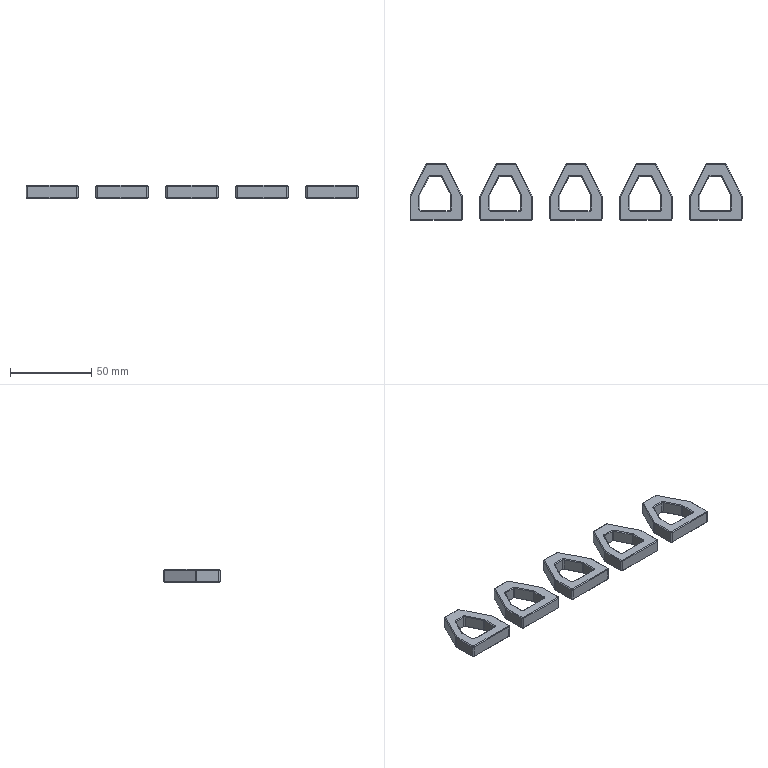NC program | NX | posted with a generic post | part box 204 x 35 x 8 mm
Whole program:
N10 G17 G21 G94 G90
(FLOOR_WALL_COPY , TOOL : D80)
N12 T19 M6
N14 G54
N16 G17 G0 G90 X-145. Y0. S6500 M3
N18 G43 Z30. H19
N20 Z4.5
N22 G94 G1 Z1.5 F1500.
N24 X-142.
N26 X142.
N28 X145.
N30 Z4.5
N32 G0 Z30.
N34 X-145.
N36 Z4.
N38 G1 Z1.
N40 X-142.
N42 X142.
N44 X145.
N46 Z4.
N48 G0 Z30.
N50 X-145.
N52 Z3.5
N54 G1 Z0.5
N56 X-142.
N58 X142.
N60 X145.
N62 Z3.5
N64 G0 Z30.
N66 X-145.
N68 Z3.
N70 G1 Z0.
N72 X-142.
N74 X142.
N76 X145.
N78 Z3.
N80 G0 Z30.
N82 M5
(PLANAR_MILL_COPY_COPY_COPY_COPY_COPY , TOOL : D6A45)
N84 T01 M6
N86 G54
N88 G17 G0 G90 X86.866 Y-19. S9500 M3
N90 G43 Z30. H1
N92 Z0.
N94 G94 G1 Z-1.5 F1250.
N96 G3 X86. Y-18.5 R1.
N98 G1 X71.
N100 G2 X69. Y-16.5 R2.
N102 G1 Y-2.736
N104 G2 X69.211 Y-1.842 R2.
N106 G1 X78.829 Y17.394
N108 G2 X80.618 Y18.5 R2.
N110 G1 X91.382
N112 G2 X93.171 Y17.394 R2.
N114 G1 X102.789 Y-1.842
N116 G2 X103. Y-2.736 R2.
N118 G1 Y-16.5
N120 G2 X101. Y-18.5 R2.
N122 G1 X86.
N124 G3 X85.134 Y-19. R1.
N126 G1 Z0.
N128 G0 Z30.
N130 X93.144 Y-1.558
N132 Z0.
N134 G1 Z-1.5
N136 G3 X93.203 Y-0.559 R1.
N138 G1 X88.674 Y8.5
N140 X82.326
N142 X77. Y-2.152
N144 Y-10.5
N146 X94.
N148 Y-2.152
N150 X93.203 Y-0.559
N152 G3 X92.369 Y-0.008 R1.
N154 G1 Z0.
N156 G0 Z30.
N158 X43.866 Y-19.
N160 Z0.
N162 G1 Z-1.5
N164 G3 X43. Y-18.5 R1.
N166 G1 X28.
N168 G2 X26. Y-16.5 R2.
N170 G1 Y-2.736
N172 G2 X26.211 Y-1.842 R2.
N174 G1 X35.829 Y17.394
N176 G2 X37.618 Y18.5 R2.
N178 G1 X48.382
N180 G2 X50.171 Y17.394 R2.
N182 G1 X59.789 Y-1.842
N184 G2 X60. Y-2.736 R2.
N186 G1 Y-16.5
N188 G2 X58. Y-18.5 R2.
N190 G1 X43.
N192 G3 X42.134 Y-19. R1.
N194 G1 Z0.
N196 G0 Z30.
N198 X50.144 Y-1.558
N200 Z0.
N202 G1 Z-1.5
N204 G3 X50.203 Y-0.559 R1.
N206 G1 X45.674 Y8.5
N208 X39.326
N210 X34. Y-2.152
N212 Y-10.5
N214 X51.
N216 Y-2.152
N218 X50.203 Y-0.559
N220 G3 X49.369 Y-0.008 R1.
N222 G1 Z0.
N224 G0 Z30.
N226 X0.866 Y-19.
N228 Z0.
N230 G1 Z-1.5
N232 G3 X0. Y-18.5 R1.
N234 G1 X-15.
N236 G2 X-17. Y-16.5 R2.
N238 G1 Y-2.736
N240 G2 X-16.789 Y-1.842 R2.
N242 G1 X-7.171 Y17.394
N244 G2 X-5.382 Y18.5 R2.
N246 G1 X5.382
N248 G2 X7.171 Y17.394 R2.
N250 G1 X16.789 Y-1.842
N252 G2 X17. Y-2.736 R2.
N254 G1 Y-16.5
N256 G2 X15. Y-18.5 R2.
N258 G1 X0.
N260 G3 X-0.866 Y-19. R1.
N262 G1 Z0.
N264 G0 Z30.
N266 X7.144 Y-1.558
N268 Z0.
N270 G1 Z-1.5
N272 G3 X7.203 Y-0.559 R1.
N274 G1 X2.674 Y8.5
N276 X-3.674
N278 X-9. Y-2.152
N280 Y-10.5
N282 X8.
N284 Y-2.152
N286 X7.203 Y-0.559
N288 G3 X6.369 Y-0.008 R1.
N290 G1 Z0.
N292 G0 Z30.
N294 X-42.134 Y-19.
N296 Z0.
N298 G1 Z-1.5
N300 G3 X-43. Y-18.5 R1.
N302 G1 X-58.
N304 G2 X-60. Y-16.5 R2.
N306 G1 Y-2.736
N308 G2 X-59.789 Y-1.842 R2.
N310 G1 X-50.171 Y17.394
N312 G2 X-48.382 Y18.5 R2.
N314 G1 X-37.618
N316 G2 X-35.829 Y17.394 R2.
N318 G1 X-26.211 Y-1.842
N320 G2 X-26. Y-2.736 R2.
N322 G1 Y-16.5
N324 G2 X-28. Y-18.5 R2.
N326 G1 X-43.
N328 G3 X-43.866 Y-19. R1.
N330 G1 Z0.
N332 G0 Z30.
N334 X-35.856 Y-1.558
N336 Z0.
N338 G1 Z-1.5
N340 G3 X-35.797 Y-0.559 R1.
N342 G1 X-40.326 Y8.5
N344 X-46.674
N346 X-52. Y-2.152
N348 Y-10.5
N350 X-35.
N352 Y-2.152
N354 X-35.797 Y-0.559
N356 G3 X-36.631 Y-0.008 R1.
N358 G1 Z0.
N360 G0 Z30.
N362 X-85.134 Y-19.
N364 Z0.
N366 G1 Z-1.5
N368 G3 X-86. Y-18.5 R1.
N370 G1 X-101.
N372 G2 X-103. Y-16.5 R2.
N374 G1 Y-2.736
N376 G2 X-102.789 Y-1.842 R2.
N378 G1 X-93.171 Y17.394
N380 G2 X-91.382 Y18.5 R2.
N382 G1 X-80.618
N384 G2 X-78.829 Y17.394 R2.
N386 G1 X-69.211 Y-1.842
N388 G2 X-69. Y-2.736 R2.
N390 G1 Y-16.5
N392 G2 X-71. Y-18.5 R2.
N394 G1 X-86.
N396 G3 X-86.866 Y-19. R1.
N398 G1 Z0.
N400 G0 Z30.
N402 X-93.369 Y-0.008
N404 Z0.
N406 G1 Z-1.5
N408 G3 X-94.203 Y-0.559 R1.
N410 G1 X-95. Y-2.152
N412 Y-10.5
N414 X-78.
N416 Y-2.152
N418 X-83.326 Y8.5
N420 X-89.674
N422 X-94.203 Y-0.559
N424 G3 X-94.144 Y-1.558 R1.
N426 G1 Z0.
N428 G0 Z30.
N430 M5
N432 M2